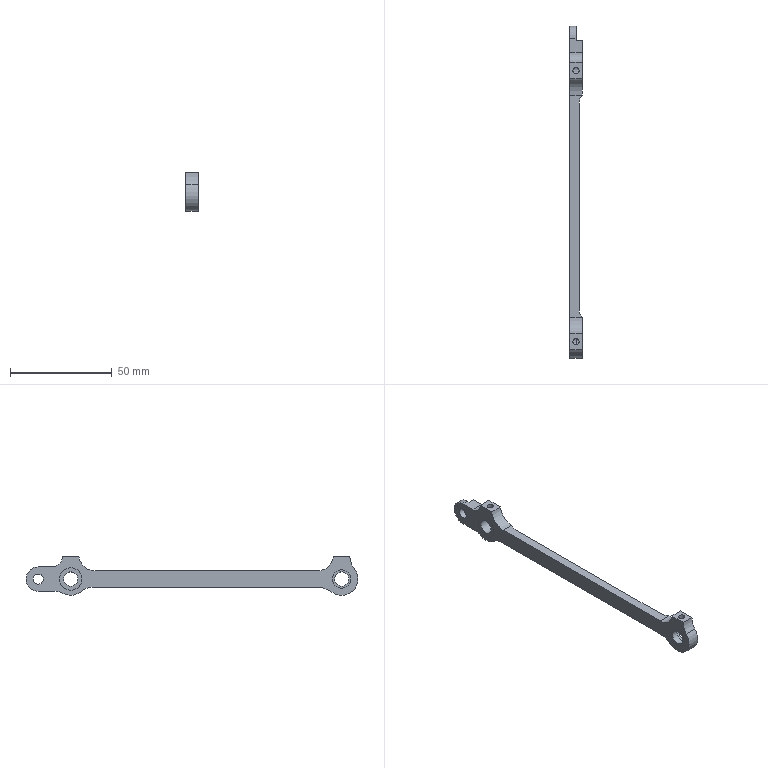Part | STEP file | COMPOUND | 3 solids | 44 faces | box 6 x 163 x 19 mm | volume 7089 mm3 | cylinder 25 | plane 19 | commonest cylinder face diameters 16 x6 3 x4 12 x4 7 x2 9 x2 11 x2